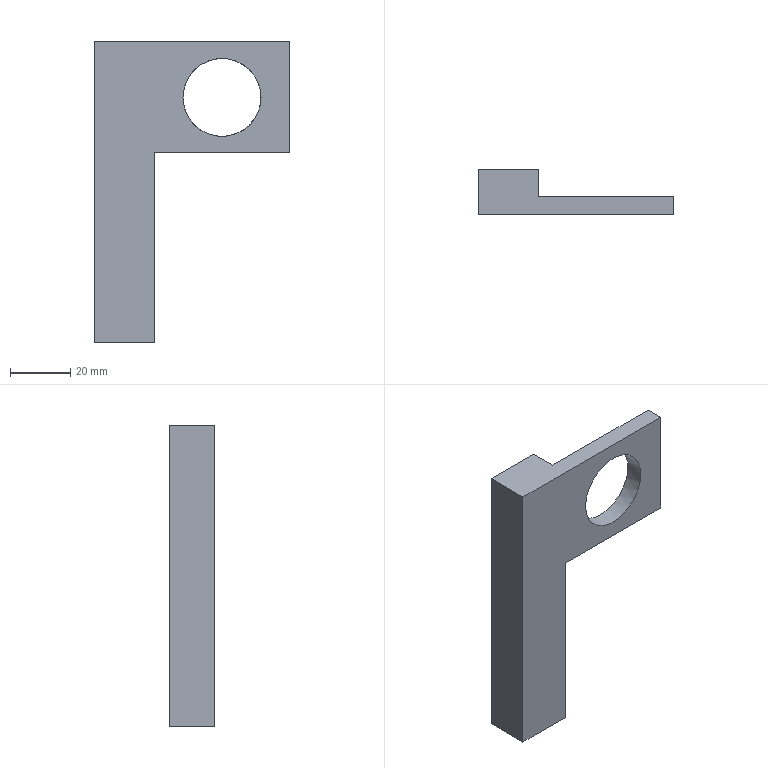Part | STEP file | Tube necking machine_id662_x_t | 1 solid | 10 faces | box 65 x 15 x 100 mm | volume 36804 mm3 | plane 9 | cylinder 1 | commonest cylinder face diameters 26 x1
STEP:
#1=CARTESIAN_POINT('',(0.,0.,0.));
#2=DIRECTION('',(0.,0.,1.));
#3=DIRECTION('',(1.,0.,0.));
#4=AXIS2_PLACEMENT_3D('',#1,#2,#3);
#5=CARTESIAN_POINT('',(240.,-166.,115.5));
#6=VERTEX_POINT('',#5);
#7=CARTESIAN_POINT('',(227.,-166.,128.5));
#8=VERTEX_POINT('',#7);
#9=CARTESIAN_POINT('',(240.,-166.,128.5));
#10=DIRECTION('',(0.,-1.,0.));
#11=DIRECTION('',(0.,0.,-1.));
#12=AXIS2_PLACEMENT_3D('',#9,#10,#11);
#13=CIRCLE('',#12,13.);
#14=CARTESIAN_POINT('',(0.,-166.,0.));
#15=DIRECTION('',(0.,-1.,0.));
#16=DIRECTION('',(0.,0.,-1.));
#17=AXIS2_PLACEMENT_3D('',#14,#15,#16);
#18=PLANE('',#17);
#19=CARTESIAN_POINT('',(-128.5,240.));
#20=DIRECTION('',(1.,0.));
#21=AXIS2_PLACEMENT_2D('',#19,#20);
#22=CIRCLE('',#21,13.);
#23=(GEOMETRIC_REPRESENTATION_CONTEXT(2)PARAMETRIC_REPRESENTATION_CONTEXT()REPRESENTATION_CONTEXT('',''));
#24=DEFINITIONAL_REPRESENTATION('',(#22),#23);
#25=PCURVE('',#18,#24);
#26=CARTESIAN_POINT('',(240.,-172.,128.5));
#27=DIRECTION('',(0.,1.,0.));
#28=DIRECTION('',(0.,0.,1.));
#29=AXIS2_PLACEMENT_3D('',#26,#27,#28);
#30=CYLINDRICAL_SURFACE('',#29,13.);
#31=CARTESIAN_POINT('',(9.425,6.));
#32=DIRECTION('',(-1.,0.));
#33=VECTOR('',#32,1.);
#34=LINE('',#31,#33);
#35=(GEOMETRIC_REPRESENTATION_CONTEXT(2)PARAMETRIC_REPRESENTATION_CONTEXT()REPRESENTATION_CONTEXT('',''));
#36=DEFINITIONAL_REPRESENTATION('',(#34),#35);
#37=PCURVE('',#30,#36);
#38=SURFACE_CURVE('',#13,(#25,#37),.PCURVE_S1.);
#39=EDGE_CURVE('',#6,#8,#38,.T.);
#40=ORIENTED_EDGE('',*,*,#39,.T.);
#41=CARTESIAN_POINT('',(240.,-166.,128.5));
#42=DIRECTION('',(0.,-1.,0.));
#43=DIRECTION('',(0.,0.,-1.));
#44=AXIS2_PLACEMENT_3D('',#41,#42,#43);
#45=CIRCLE('',#44,13.);
#46=CARTESIAN_POINT('',(-128.5,240.));
#47=DIRECTION('',(1.,0.));
#48=AXIS2_PLACEMENT_2D('',#46,#47);
#49=CIRCLE('',#48,13.);
#50=(GEOMETRIC_REPRESENTATION_CONTEXT(2)PARAMETRIC_REPRESENTATION_CONTEXT()REPRESENTATION_CONTEXT('',''));
#51=DEFINITIONAL_REPRESENTATION('',(#49),#50);
#52=PCURVE('',#18,#51);
#53=CARTESIAN_POINT('',(15.708,6.));
#54=DIRECTION('',(-1.,0.));
#55=VECTOR('',#54,1.);
#56=LINE('',#53,#55);
#57=(GEOMETRIC_REPRESENTATION_CONTEXT(2)PARAMETRIC_REPRESENTATION_CONTEXT()REPRESENTATION_CONTEXT('',''));
#58=DEFINITIONAL_REPRESENTATION('',(#56),#57);
#59=PCURVE('',#30,#58);
#60=SURFACE_CURVE('',#45,(#52,#59),.PCURVE_S1.);
#61=EDGE_CURVE('',#8,#6,#60,.T.);
#62=ORIENTED_EDGE('',*,*,#61,.T.);
#63=EDGE_LOOP('',(#40,#62));
#64=FACE_BOUND('',#63,.T.);
#65=CARTESIAN_POINT('',(217.5,-166.,147.));
#66=VERTEX_POINT('',#65);
#67=CARTESIAN_POINT('',(217.5,-166.,110.));
#68=VERTEX_POINT('',#67);
#69=CARTESIAN_POINT('',(217.5,-166.,0.));
#70=DIRECTION('',(0.,0.,-1.));
#71=VECTOR('',#70,1.);
#72=LINE('',#69,#71);
#73=CARTESIAN_POINT('',(0.,217.5));
#74=DIRECTION('',(1.,0.));
#75=VECTOR('',#74,1.);
#76=LINE('',#73,#75);
#77=(GEOMETRIC_REPRESENTATION_CONTEXT(2)PARAMETRIC_REPRESENTATION_CONTEXT()REPRESENTATION_CONTEXT('',''));
#78=DEFINITIONAL_REPRESENTATION('',(#76),#77);
#79=PCURVE('',#18,#78);
#80=CARTESIAN_POINT('',(217.5,-166.,47.));
#81=DIRECTION('',(1.,0.,0.));
#82=DIRECTION('',(0.,0.,-1.));
#83=AXIS2_PLACEMENT_3D('',#80,#81,#82);
#84=PLANE('',#83);
#85=CARTESIAN_POINT('',(47.,0.));
#86=DIRECTION('',(1.,0.));
#87=VECTOR('',#86,1.);
#88=LINE('',#85,#87);
#89=(GEOMETRIC_REPRESENTATION_CONTEXT(2)PARAMETRIC_REPRESENTATION_CONTEXT()REPRESENTATION_CONTEXT('',''));
#90=DEFINITIONAL_REPRESENTATION('',(#88),#89);
#91=PCURVE('',#84,#90);
#92=SURFACE_CURVE('',#72,(#79,#91),.PCURVE_S1.);
#93=EDGE_CURVE('',#66,#68,#92,.T.);
#94=ORIENTED_EDGE('',*,*,#93,.F.);
#95=CARTESIAN_POINT('',(262.5,-166.,147.));
#96=VERTEX_POINT('',#95);
#97=CARTESIAN_POINT('',(262.5,-166.,147.));
#98=DIRECTION('',(-1.,0.,0.));
#99=VECTOR('',#98,1.);
#100=LINE('',#97,#99);
#101=CARTESIAN_POINT('',(-147.,262.5));
#102=DIRECTION('',(0.,-1.));
#103=VECTOR('',#102,1.);
#104=LINE('',#101,#103);
#105=(GEOMETRIC_REPRESENTATION_CONTEXT(2)PARAMETRIC_REPRESENTATION_CONTEXT()REPRESENTATION_CONTEXT('',''));
#106=DEFINITIONAL_REPRESENTATION('',(#104),#105);
#107=PCURVE('',#18,#106);
#108=CARTESIAN_POINT('',(262.5,-166.,147.));
#109=DIRECTION('',(0.,0.,1.));
#110=DIRECTION('',(1.,0.,0.));
#111=AXIS2_PLACEMENT_3D('',#108,#109,#110);
#112=PLANE('',#111);
#113=CARTESIAN_POINT('',(0.,0.));
#114=DIRECTION('',(-1.,0.));
#115=VECTOR('',#114,1.);
#116=LINE('',#113,#115);
#117=(GEOMETRIC_REPRESENTATION_CONTEXT(2)PARAMETRIC_REPRESENTATION_CONTEXT()REPRESENTATION_CONTEXT('',''));
#118=DEFINITIONAL_REPRESENTATION('',(#116),#117);
#119=PCURVE('',#112,#118);
#120=SURFACE_CURVE('',#100,(#107,#119),.PCURVE_S1.);
#121=EDGE_CURVE('',#96,#66,#120,.T.);
#122=ORIENTED_EDGE('',*,*,#121,.F.);
#123=CARTESIAN_POINT('',(262.5,-166.,110.));
#124=VERTEX_POINT('',#123);
#125=CARTESIAN_POINT('',(262.5,-166.,110.));
#126=DIRECTION('',(0.,0.,1.));
#127=VECTOR('',#126,1.);
#128=LINE('',#125,#127);
#129=CARTESIAN_POINT('',(-110.,262.5));
#130=DIRECTION('',(-1.,0.));
#131=VECTOR('',#130,1.);
#132=LINE('',#129,#131);
#133=(GEOMETRIC_REPRESENTATION_CONTEXT(2)PARAMETRIC_REPRESENTATION_CONTEXT()REPRESENTATION_CONTEXT('',''));
#134=DEFINITIONAL_REPRESENTATION('',(#132),#133);
#135=PCURVE('',#18,#134);
#136=CARTESIAN_POINT('',(262.5,-166.,110.));
#137=DIRECTION('',(1.,0.,0.));
#138=DIRECTION('',(0.,0.,-1.));
#139=AXIS2_PLACEMENT_3D('',#136,#137,#138);
#140=PLANE('',#139);
#141=CARTESIAN_POINT('',(0.,0.));
#142=DIRECTION('',(-1.,0.));
#143=VECTOR('',#142,1.);
#144=LINE('',#141,#143);
#145=(GEOMETRIC_REPRESENTATION_CONTEXT(2)PARAMETRIC_REPRESENTATION_CONTEXT()REPRESENTATION_CONTEXT('',''));
#146=DEFINITIONAL_REPRESENTATION('',(#144),#145);
#147=PCURVE('',#140,#146);
#148=SURFACE_CURVE('',#128,(#135,#147),.PCURVE_S1.);
#149=EDGE_CURVE('',#124,#96,#148,.T.);
#150=ORIENTED_EDGE('',*,*,#149,.F.);
#151=CARTESIAN_POINT('',(217.5,-166.,110.));
#152=DIRECTION('',(1.,0.,0.));
#153=VECTOR('',#152,1.);
#154=LINE('',#151,#153);
#155=CARTESIAN_POINT('',(-110.,217.5));
#156=DIRECTION('',(0.,1.));
#157=VECTOR('',#156,1.);
#158=LINE('',#155,#157);
#159=(GEOMETRIC_REPRESENTATION_CONTEXT(2)PARAMETRIC_REPRESENTATION_CONTEXT()REPRESENTATION_CONTEXT('',''));
#160=DEFINITIONAL_REPRESENTATION('',(#158),#159);
#161=PCURVE('',#18,#160);
#162=CARTESIAN_POINT('',(217.5,-166.,110.));
#163=DIRECTION('',(0.,0.,-1.));
#164=DIRECTION('',(-1.,0.,0.));
#165=AXIS2_PLACEMENT_3D('',#162,#163,#164);
#166=PLANE('',#165);
#167=CARTESIAN_POINT('',(0.,0.));
#168=DIRECTION('',(-1.,0.));
#169=VECTOR('',#168,1.);
#170=LINE('',#167,#169);
#171=(GEOMETRIC_REPRESENTATION_CONTEXT(2)PARAMETRIC_REPRESENTATION_CONTEXT()REPRESENTATION_CONTEXT('',''));
#172=DEFINITIONAL_REPRESENTATION('',(#170),#171);
#173=PCURVE('',#166,#172);
#174=SURFACE_CURVE('',#154,(#161,#173),.PCURVE_S1.);
#175=EDGE_CURVE('',#68,#124,#174,.T.);
#176=ORIENTED_EDGE('',*,*,#175,.F.);
#177=EDGE_LOOP('',(#94,#122,#150,#176));
#178=FACE_BOUND('',#177,.T.);
#179=ADVANCED_FACE('',(#64,#178),#18,.F.);
#180=CARTESIAN_POINT('',(197.5,-172.,147.));
#181=VERTEX_POINT('',#180);
#182=CARTESIAN_POINT('',(197.5,-172.,47.));
#183=VERTEX_POINT('',#182);
#184=CARTESIAN_POINT('',(197.5,-172.,147.));
#185=DIRECTION('',(0.,0.,-1.));
#186=VECTOR('',#185,1.);
#187=LINE('',#184,#186);
#188=CARTESIAN_POINT('',(197.5,-166.,147.));
#189=DIRECTION('',(-1.,0.,0.));
#190=DIRECTION('',(0.,0.,1.));
#191=AXIS2_PLACEMENT_3D('',#188,#189,#190);
#192=PLANE('',#191);
#193=CARTESIAN_POINT('',(0.,-6.));
#194=DIRECTION('',(-1.,0.));
#195=VECTOR('',#194,1.);
#196=LINE('',#193,#195);
#197=(GEOMETRIC_REPRESENTATION_CONTEXT(2)PARAMETRIC_REPRESENTATION_CONTEXT()REPRESENTATION_CONTEXT('',''));
#198=DEFINITIONAL_REPRESENTATION('',(#196),#197);
#199=PCURVE('',#192,#198);
#200=CARTESIAN_POINT('',(0.,-172.,0.));
#201=DIRECTION('',(0.,-1.,0.));
#202=DIRECTION('',(0.,0.,-1.));
#203=AXIS2_PLACEMENT_3D('',#200,#201,#202);
#204=PLANE('',#203);
#205=CARTESIAN_POINT('',(-147.,197.5));
#206=DIRECTION('',(1.,0.));
#207=VECTOR('',#206,1.);
#208=LINE('',#205,#207);
#209=(GEOMETRIC_REPRESENTATION_CONTEXT(2)PARAMETRIC_REPRESENTATION_CONTEXT()REPRESENTATION_CONTEXT('',''));
#210=DEFINITIONAL_REPRESENTATION('',(#208),#209);
#211=PCURVE('',#204,#210);
#212=SURFACE_CURVE('',#187,(#199,#211),.PCURVE_S1.);
#213=EDGE_CURVE('',#181,#183,#212,.T.);
#214=ORIENTED_EDGE('',*,*,#213,.F.);
#215=CARTESIAN_POINT('',(197.5,-157.,147.));
#216=VERTEX_POINT('',#215);
#217=CARTESIAN_POINT('',(197.5,-166.,147.));
#218=DIRECTION('',(0.,-1.,0.));
#219=VECTOR('',#218,1.);
#220=LINE('',#217,#219);
#221=CARTESIAN_POINT('',(0.,0.));
#222=DIRECTION('',(0.,-1.));
#223=VECTOR('',#222,1.);
#224=LINE('',#221,#223);
#225=(GEOMETRIC_REPRESENTATION_CONTEXT(2)PARAMETRIC_REPRESENTATION_CONTEXT()REPRESENTATION_CONTEXT('',''));
#226=DEFINITIONAL_REPRESENTATION('',(#224),#225);
#227=PCURVE('',#192,#226);
#228=CARTESIAN_POINT('',(-65.,0.));
#229=DIRECTION('',(0.,-1.));
#230=VECTOR('',#229,1.);
#231=LINE('',#228,#230);
#232=(GEOMETRIC_REPRESENTATION_CONTEXT(2)PARAMETRIC_REPRESENTATION_CONTEXT()REPRESENTATION_CONTEXT('',''));
#233=DEFINITIONAL_REPRESENTATION('',(#231),#232);
#234=PCURVE('',#112,#233);
#235=SURFACE_CURVE('',#220,(#227,#234),.PCURVE_S1.);
#236=EDGE_CURVE('',#216,#181,#235,.T.);
#237=ORIENTED_EDGE('',*,*,#236,.F.);
#238=CARTESIAN_POINT('',(197.5,-157.,47.));
#239=VERTEX_POINT('',#238);
#240=CARTESIAN_POINT('',(197.5,-157.,147.));
#241=DIRECTION('',(0.,0.,-1.));
#242=VECTOR('',#241,1.);
#243=LINE('',#240,#242);
#244=CARTESIAN_POINT('',(0.,9.));
#245=DIRECTION('',(-1.,0.));
#246=VECTOR('',#245,1.);
#247=LINE('',#244,#246);
#248=(GEOMETRIC_REPRESENTATION_CONTEXT(2)PARAMETRIC_REPRESENTATION_CONTEXT()REPRESENTATION_CONTEXT('',''));
#249=DEFINITIONAL_REPRESENTATION('',(#247),#248);
#250=PCURVE('',#192,#249);
#251=CARTESIAN_POINT('',(197.5,-157.,147.));
#252=DIRECTION('',(0.,1.,0.));
#253=DIRECTION('',(0.,0.,-1.));
#254=AXIS2_PLACEMENT_3D('',#251,#252,#253);
#255=PLANE('',#254);
#256=CARTESIAN_POINT('',(0.,0.));
#257=DIRECTION('',(1.,0.));
#258=VECTOR('',#257,1.);
#259=LINE('',#256,#258);
#260=(GEOMETRIC_REPRESENTATION_CONTEXT(2)PARAMETRIC_REPRESENTATION_CONTEXT()REPRESENTATION_CONTEXT('',''));
#261=DEFINITIONAL_REPRESENTATION('',(#259),#260);
#262=PCURVE('',#255,#261);
#263=SURFACE_CURVE('',#243,(#250,#262),.PCURVE_S1.);
#264=EDGE_CURVE('',#216,#239,#263,.T.);
#265=ORIENTED_EDGE('',*,*,#264,.T.);
#266=CARTESIAN_POINT('',(197.5,-166.,47.));
#267=DIRECTION('',(0.,-1.,0.));
#268=VECTOR('',#267,1.);
#269=LINE('',#266,#268);
#270=CARTESIAN_POINT('',(-100.,0.));
#271=DIRECTION('',(0.,-1.));
#272=VECTOR('',#271,1.);
#273=LINE('',#270,#272);
#274=(GEOMETRIC_REPRESENTATION_CONTEXT(2)PARAMETRIC_REPRESENTATION_CONTEXT()REPRESENTATION_CONTEXT('',''));
#275=DEFINITIONAL_REPRESENTATION('',(#273),#274);
#276=PCURVE('',#192,#275);
#277=CARTESIAN_POINT('',(197.5,-166.,47.));
#278=DIRECTION('',(0.,0.,-1.));
#279=DIRECTION('',(-1.,0.,0.));
#280=AXIS2_PLACEMENT_3D('',#277,#278,#279);
#281=PLANE('',#280);
#282=CARTESIAN_POINT('',(0.,0.));
#283=DIRECTION('',(0.,-1.));
#284=VECTOR('',#283,1.);
#285=LINE('',#282,#284);
#286=(GEOMETRIC_REPRESENTATION_CONTEXT(2)PARAMETRIC_REPRESENTATION_CONTEXT()REPRESENTATION_CONTEXT('',''));
#287=DEFINITIONAL_REPRESENTATION('',(#285),#286);
#288=PCURVE('',#281,#287);
#289=SURFACE_CURVE('',#269,(#276,#288),.PCURVE_S1.);
#290=EDGE_CURVE('',#239,#183,#289,.T.);
#291=ORIENTED_EDGE('',*,*,#290,.T.);
#292=EDGE_LOOP('',(#214,#237,#265,#291));
#293=FACE_BOUND('',#292,.T.);
#294=ADVANCED_FACE('',(#293),#192,.T.);
#295=CARTESIAN_POINT('',(217.5,-172.,47.));
#296=VERTEX_POINT('',#295);
#297=CARTESIAN_POINT('',(197.5,-172.,47.));
#298=DIRECTION('',(1.,0.,0.));
#299=VECTOR('',#298,1.);
#300=LINE('',#297,#299);
#301=CARTESIAN_POINT('',(0.,-6.));
#302=DIRECTION('',(-1.,0.));
#303=VECTOR('',#302,1.);
#304=LINE('',#301,#303);
#305=(GEOMETRIC_REPRESENTATION_CONTEXT(2)PARAMETRIC_REPRESENTATION_CONTEXT()REPRESENTATION_CONTEXT('',''));
#306=DEFINITIONAL_REPRESENTATION('',(#304),#305);
#307=PCURVE('',#281,#306);
#308=CARTESIAN_POINT('',(-47.,197.5));
#309=DIRECTION('',(0.,1.));
#310=VECTOR('',#309,1.);
#311=LINE('',#308,#310);
#312=(GEOMETRIC_REPRESENTATION_CONTEXT(2)PARAMETRIC_REPRESENTATION_CONTEXT()REPRESENTATION_CONTEXT('',''));
#313=DEFINITIONAL_REPRESENTATION('',(#311),#312);
#314=PCURVE('',#204,#313);
#315=SURFACE_CURVE('',#300,(#307,#314),.PCURVE_S1.);
#316=EDGE_CURVE('',#183,#296,#315,.T.);
#317=ORIENTED_EDGE('',*,*,#316,.F.);
#318=ORIENTED_EDGE('',*,*,#290,.F.);
#319=CARTESIAN_POINT('',(217.5,-157.,47.));
#320=VERTEX_POINT('',#319);
#321=CARTESIAN_POINT('',(197.5,-157.,47.));
#322=DIRECTION('',(1.,0.,0.));
#323=VECTOR('',#322,1.);
#324=LINE('',#321,#323);
#325=CARTESIAN_POINT('',(0.,9.));
#326=DIRECTION('',(-1.,0.));
#327=VECTOR('',#326,1.);
#328=LINE('',#325,#327);
#329=(GEOMETRIC_REPRESENTATION_CONTEXT(2)PARAMETRIC_REPRESENTATION_CONTEXT()REPRESENTATION_CONTEXT('',''));
#330=DEFINITIONAL_REPRESENTATION('',(#328),#329);
#331=PCURVE('',#281,#330);
#332=CARTESIAN_POINT('',(100.,0.));
#333=DIRECTION('',(0.,-1.));
#334=VECTOR('',#333,1.);
#335=LINE('',#332,#334);
#336=(GEOMETRIC_REPRESENTATION_CONTEXT(2)PARAMETRIC_REPRESENTATION_CONTEXT()REPRESENTATION_CONTEXT('',''));
#337=DEFINITIONAL_REPRESENTATION('',(#335),#336);
#338=PCURVE('',#255,#337);
#339=SURFACE_CURVE('',#324,(#331,#338),.PCURVE_S1.);
#340=EDGE_CURVE('',#239,#320,#339,.T.);
#341=ORIENTED_EDGE('',*,*,#340,.T.);
#342=CARTESIAN_POINT('',(217.5,-166.,47.));
#343=DIRECTION('',(0.,-1.,0.));
#344=VECTOR('',#343,1.);
#345=LINE('',#342,#344);
#346=CARTESIAN_POINT('',(-20.,0.));
#347=DIRECTION('',(0.,-1.));
#348=VECTOR('',#347,1.);
#349=LINE('',#346,#348);
#350=(GEOMETRIC_REPRESENTATION_CONTEXT(2)PARAMETRIC_REPRESENTATION_CONTEXT()REPRESENTATION_CONTEXT('',''));
#351=DEFINITIONAL_REPRESENTATION('',(#349),#350);
#352=PCURVE('',#281,#351);
#353=CARTESIAN_POINT('',(0.,0.));
#354=DIRECTION('',(0.,-1.));
#355=VECTOR('',#354,1.);
#356=LINE('',#353,#355);
#357=(GEOMETRIC_REPRESENTATION_CONTEXT(2)PARAMETRIC_REPRESENTATION_CONTEXT()REPRESENTATION_CONTEXT('',''));
#358=DEFINITIONAL_REPRESENTATION('',(#356),#357);
#359=PCURVE('',#84,#358);
#360=SURFACE_CURVE('',#345,(#352,#359),.PCURVE_S1.);
#361=EDGE_CURVE('',#320,#296,#360,.T.);
#362=ORIENTED_EDGE('',*,*,#361,.T.);
#363=EDGE_LOOP('',(#317,#318,#341,#362));
#364=FACE_BOUND('',#363,.T.);
#365=ADVANCED_FACE('',(#364),#281,.T.);
#366=CARTESIAN_POINT('',(217.5,-172.,110.));
#367=VERTEX_POINT('',#366);
#368=CARTESIAN_POINT('',(217.5,-172.,47.));
#369=DIRECTION('',(0.,0.,1.));
#370=VECTOR('',#369,1.);
#371=LINE('',#368,#370);
#372=CARTESIAN_POINT('',(0.,-6.));
#373=DIRECTION('',(-1.,0.));
#374=VECTOR('',#373,1.);
#375=LINE('',#372,#374);
#376=(GEOMETRIC_REPRESENTATION_CONTEXT(2)PARAMETRIC_REPRESENTATION_CONTEXT()REPRESENTATION_CONTEXT('',''));
#377=DEFINITIONAL_REPRESENTATION('',(#375),#376);
#378=PCURVE('',#84,#377);
#379=CARTESIAN_POINT('',(-47.,217.5));
#380=DIRECTION('',(-1.,0.));
#381=VECTOR('',#380,1.);
#382=LINE('',#379,#381);
#383=(GEOMETRIC_REPRESENTATION_CONTEXT(2)PARAMETRIC_REPRESENTATION_CONTEXT()REPRESENTATION_CONTEXT('',''));
#384=DEFINITIONAL_REPRESENTATION('',(#382),#383);
#385=PCURVE('',#204,#384);
#386=SURFACE_CURVE('',#371,(#378,#385),.PCURVE_S1.);
#387=EDGE_CURVE('',#296,#367,#386,.T.);
#388=ORIENTED_EDGE('',*,*,#387,.F.);
#389=ORIENTED_EDGE('',*,*,#361,.F.);
#390=CARTESIAN_POINT('',(217.5,-157.,147.));
#391=VERTEX_POINT('',#390);
#392=CARTESIAN_POINT('',(217.5,-157.,147.));
#393=DIRECTION('',(0.,0.,-1.));
#394=VECTOR('',#393,1.);
#395=LINE('',#392,#394);
#396=CARTESIAN_POINT('',(-100.,9.));
#397=DIRECTION('',(1.,0.));
#398=VECTOR('',#397,1.);
#399=LINE('',#396,#398);
#400=(GEOMETRIC_REPRESENTATION_CONTEXT(2)PARAMETRIC_REPRESENTATION_CONTEXT()REPRESENTATION_CONTEXT('',''));
#401=DEFINITIONAL_REPRESENTATION('',(#399),#400);
#402=PCURVE('',#84,#401);
#403=CARTESIAN_POINT('',(0.,-20.));
#404=DIRECTION('',(1.,0.));
#405=VECTOR('',#404,1.);
#406=LINE('',#403,#405);
#407=(GEOMETRIC_REPRESENTATION_CONTEXT(2)PARAMETRIC_REPRESENTATION_CONTEXT()REPRESENTATION_CONTEXT('',''));
#408=DEFINITIONAL_REPRESENTATION('',(#406),#407);
#409=PCURVE('',#255,#408);
#410=SURFACE_CURVE('',#395,(#402,#409),.PCURVE_S1.);
#411=EDGE_CURVE('',#391,#320,#410,.T.);
#412=ORIENTED_EDGE('',*,*,#411,.F.);
#413=CARTESIAN_POINT('',(217.5,-157.,147.));
#414=DIRECTION('',(0.,-1.,0.));
#415=VECTOR('',#414,1.);
#416=LINE('',#413,#415);
#417=CARTESIAN_POINT('',(-100.,9.));
#418=DIRECTION('',(0.,-1.));
#419=VECTOR('',#418,1.);
#420=LINE('',#417,#419);
#421=(GEOMETRIC_REPRESENTATION_CONTEXT(2)PARAMETRIC_REPRESENTATION_CONTEXT()REPRESENTATION_CONTEXT('',''));
#422=DEFINITIONAL_REPRESENTATION('',(#420),#421);
#423=PCURVE('',#84,#422);
#424=CARTESIAN_POINT('',(-45.,9.));
#425=DIRECTION('',(0.,-1.));
#426=VECTOR('',#425,1.);
#427=LINE('',#424,#426);
#428=(GEOMETRIC_REPRESENTATION_CONTEXT(2)PARAMETRIC_REPRESENTATION_CONTEXT()REPRESENTATION_CONTEXT('',''));
#429=DEFINITIONAL_REPRESENTATION('',(#427),#428);
#430=PCURVE('',#112,#429);
#431=SURFACE_CURVE('',#416,(#423,#430),.PCURVE_S1.);
#432=EDGE_CURVE('',#391,#66,#431,.T.);
#433=ORIENTED_EDGE('',*,*,#432,.T.);
#434=ORIENTED_EDGE('',*,*,#93,.T.);
#435=CARTESIAN_POINT('',(217.5,-166.,110.));
#436=DIRECTION('',(0.,-1.,0.));
#437=VECTOR('',#436,1.);
#438=LINE('',#435,#437);
#439=CARTESIAN_POINT('',(-63.,0.));
#440=DIRECTION('',(0.,-1.));
#441=VECTOR('',#440,1.);
#442=LINE('',#439,#441);
#443=(GEOMETRIC_REPRESENTATION_CONTEXT(2)PARAMETRIC_REPRESENTATION_CONTEXT()REPRESENTATION_CONTEXT('',''));
#444=DEFINITIONAL_REPRESENTATION('',(#442),#443);
#445=PCURVE('',#84,#444);
#446=CARTESIAN_POINT('',(0.,0.));
#447=DIRECTION('',(0.,-1.));
#448=VECTOR('',#447,1.);
#449=LINE('',#446,#448);
#450=(GEOMETRIC_REPRESENTATION_CONTEXT(2)PARAMETRIC_REPRESENTATION_CONTEXT()REPRESENTATION_CONTEXT('',''));
#451=DEFINITIONAL_REPRESENTATION('',(#449),#450);
#452=PCURVE('',#166,#451);
#453=SURFACE_CURVE('',#438,(#445,#452),.PCURVE_S1.);
#454=EDGE_CURVE('',#68,#367,#453,.T.);
#455=ORIENTED_EDGE('',*,*,#454,.T.);
#456=EDGE_LOOP('',(#388,#389,#412,#433,#434,#455));
#457=FACE_BOUND('',#456,.T.);
#458=ADVANCED_FACE('',(#457),#84,.T.);
#459=CARTESIAN_POINT('',(262.5,-172.,110.));
#460=VERTEX_POINT('',#459);
#461=CARTESIAN_POINT('',(217.5,-172.,110.));
#462=DIRECTION('',(1.,0.,0.));
#463=VECTOR('',#462,1.);
#464=LINE('',#461,#463);
#465=CARTESIAN_POINT('',(0.,-6.));
#466=DIRECTION('',(-1.,0.));
#467=VECTOR('',#466,1.);
#468=LINE('',#465,#467);
#469=(GEOMETRIC_REPRESENTATION_CONTEXT(2)PARAMETRIC_REPRESENTATION_CONTEXT()REPRESENTATION_CONTEXT('',''));
#470=DEFINITIONAL_REPRESENTATION('',(#468),#469);
#471=PCURVE('',#166,#470);
#472=CARTESIAN_POINT('',(-110.,217.5));
#473=DIRECTION('',(0.,1.));
#474=VECTOR('',#473,1.);
#475=LINE('',#472,#474);
#476=(GEOMETRIC_REPRESENTATION_CONTEXT(2)PARAMETRIC_REPRESENTATION_CONTEXT()REPRESENTATION_CONTEXT('',''));
#477=DEFINITIONAL_REPRESENTATION('',(#475),#476);
#478=PCURVE('',#204,#477);
#479=SURFACE_CURVE('',#464,(#471,#478),.PCURVE_S1.);
#480=EDGE_CURVE('',#367,#460,#479,.T.);
#481=ORIENTED_EDGE('',*,*,#480,.F.);
#482=ORIENTED_EDGE('',*,*,#454,.F.);
#483=ORIENTED_EDGE('',*,*,#175,.T.);
#484=CARTESIAN_POINT('',(262.5,-166.,110.));
#485=DIRECTION('',(0.,-1.,0.));
#486=VECTOR('',#485,1.);
#487=LINE('',#484,#486);
#488=CARTESIAN_POINT('',(-45.,0.));
#489=DIRECTION('',(0.,-1.));
#490=VECTOR('',#489,1.);
#491=LINE('',#488,#490);
#492=(GEOMETRIC_REPRESENTATION_CONTEXT(2)PARAMETRIC_REPRESENTATION_CONTEXT()REPRESENTATION_CONTEXT('',''));
#493=DEFINITIONAL_REPRESENTATION('',(#491),#492);
#494=PCURVE('',#166,#493);
#495=CARTESIAN_POINT('',(0.,0.));
#496=DIRECTION('',(0.,-1.));
#497=VECTOR('',#496,1.);
#498=LINE('',#495,#497);
#499=(GEOMETRIC_REPRESENTATION_CONTEXT(2)PARAMETRIC_REPRESENTATION_CONTEXT()REPRESENTATION_CONTEXT('',''));
#500=DEFINITIONAL_REPRESENTATION('',(#498),#499);
#501=PCURVE('',#140,#500);
#502=SURFACE_CURVE('',#487,(#494,#501),.PCURVE_S1.);
#503=EDGE_CURVE('',#124,#460,#502,.T.);
#504=ORIENTED_EDGE('',*,*,#503,.T.);
#505=EDGE_LOOP('',(#481,#482,#483,#504));
#506=FACE_BOUND('',#505,.T.);
#507=ADVANCED_FACE('',(#506),#166,.T.);
#508=CARTESIAN_POINT('',(262.5,-172.,147.));
#509=VERTEX_POINT('',#508);
#510=CARTESIAN_POINT('',(262.5,-172.,110.));
#511=DIRECTION('',(0.,0.,1.));
#512=VECTOR('',#511,1.);
#513=LINE('',#510,#512);
#514=CARTESIAN_POINT('',(0.,-6.));
#515=DIRECTION('',(-1.,0.));
#516=VECTOR('',#515,1.);
#517=LINE('',#514,#516);
#518=(GEOMETRIC_REPRESENTATION_CONTEXT(2)PARAMETRIC_REPRESENTATION_CONTEXT()REPRESENTATION_CONTEXT('',''));
#519=DEFINITIONAL_REPRESENTATION('',(#517),#518);
#520=PCURVE('',#140,#519);
#521=CARTESIAN_POINT('',(-110.,262.5));
#522=DIRECTION('',(-1.,0.));
#523=VECTOR('',#522,1.);
#524=LINE('',#521,#523);
#525=(GEOMETRIC_REPRESENTATION_CONTEXT(2)PARAMETRIC_REPRESENTATION_CONTEXT()REPRESENTATION_CONTEXT('',''));
#526=DEFINITIONAL_REPRESENTATION('',(#524),#525);
#527=PCURVE('',#204,#526);
#528=SURFACE_CURVE('',#513,(#520,#527),.PCURVE_S1.);
#529=EDGE_CURVE('',#460,#509,#528,.T.);
#530=ORIENTED_EDGE('',*,*,#529,.F.);
#531=ORIENTED_EDGE('',*,*,#503,.F.);
#532=ORIENTED_EDGE('',*,*,#149,.T.);
#533=CARTESIAN_POINT('',(262.5,-166.,147.));
#534=DIRECTION('',(0.,-1.,0.));
#535=VECTOR('',#534,1.);
#536=LINE('',#533,#535);
#537=CARTESIAN_POINT('',(-37.,0.));
#538=DIRECTION('',(0.,-1.));
#539=VECTOR('',#538,1.);
#540=LINE('',#537,#539);
#541=(GEOMETRIC_REPRESENTATION_CONTEXT(2)PARAMETRIC_REPRESENTATION_CONTEXT()REPRESENTATION_CONTEXT('',''));
#542=DEFINITIONAL_REPRESENTATION('',(#540),#541);
#543=PCURVE('',#140,#542);
#544=CARTESIAN_POINT('',(0.,0.));
#545=DIRECTION('',(0.,-1.));
#546=VECTOR('',#545,1.);
#547=LINE('',#544,#546);
#548=(GEOMETRIC_REPRESENTATION_CONTEXT(2)PARAMETRIC_REPRESENTATION_CONTEXT()REPRESENTATION_CONTEXT('',''));
#549=DEFINITIONAL_REPRESENTATION('',(#547),#548);
#550=PCURVE('',#112,#549);
#551=SURFACE_CURVE('',#536,(#543,#550),.PCURVE_S1.);
#552=EDGE_CURVE('',#96,#509,#551,.T.);
#553=ORIENTED_EDGE('',*,*,#552,.T.);
#554=EDGE_LOOP('',(#530,#531,#532,#553));
#555=FACE_BOUND('',#554,.T.);
#556=ADVANCED_FACE('',(#555),#140,.T.);
#557=ORIENTED_EDGE('',*,*,#236,.T.);
#558=CARTESIAN_POINT('',(262.5,-172.,147.));
#559=DIRECTION('',(-1.,0.,0.));
#560=VECTOR('',#559,1.);
#561=LINE('',#558,#560);
#562=CARTESIAN_POINT('',(0.,-6.));
#563=DIRECTION('',(-1.,0.));
#564=VECTOR('',#563,1.);
#565=LINE('',#562,#564);
#566=(GEOMETRIC_REPRESENTATION_CONTEXT(2)PARAMETRIC_REPRESENTATION_CONTEXT()REPRESENTATION_CONTEXT('',''));
#567=DEFINITIONAL_REPRESENTATION('',(#565),#566);
#568=PCURVE('',#112,#567);
#569=CARTESIAN_POINT('',(-147.,262.5));
#570=DIRECTION('',(0.,-1.));
#571=VECTOR('',#570,1.);
#572=LINE('',#569,#571);
#573=(GEOMETRIC_REPRESENTATION_CONTEXT(2)PARAMETRIC_REPRESENTATION_CONTEXT()REPRESENTATION_CONTEXT('',''));
#574=DEFINITIONAL_REPRESENTATION('',(#572),#573);
#575=PCURVE('',#204,#574);
#576=SURFACE_CURVE('',#561,(#568,#575),.PCURVE_S1.);
#577=EDGE_CURVE('',#509,#181,#576,.T.);
#578=ORIENTED_EDGE('',*,*,#577,.F.);
#579=ORIENTED_EDGE('',*,*,#552,.F.);
#580=ORIENTED_EDGE('',*,*,#121,.T.);
#581=ORIENTED_EDGE('',*,*,#432,.F.);
#582=CARTESIAN_POINT('',(197.5,-157.,147.));
#583=DIRECTION('',(1.,0.,0.));
#584=VECTOR('',#583,1.);
#585=LINE('',#582,#584);
#586=CARTESIAN_POINT('',(-65.,9.));
#587=DIRECTION('',(1.,0.));
#588=VECTOR('',#587,1.);
#589=LINE('',#586,#588);
#590=(GEOMETRIC_REPRESENTATION_CONTEXT(2)PARAMETRIC_REPRESENTATION_CONTEXT()REPRESENTATION_CONTEXT('',''));
#591=DEFINITIONAL_REPRESENTATION('',(#589),#590);
#592=PCURVE('',#112,#591);
#593=CARTESIAN_POINT('',(0.,0.));
#594=DIRECTION('',(0.,-1.));
#595=VECTOR('',#594,1.);
#596=LINE('',#593,#595);
#597=(GEOMETRIC_REPRESENTATION_CONTEXT(2)PARAMETRIC_REPRESENTATION_CONTEXT()REPRESENTATION_CONTEXT('',''));
#598=DEFINITIONAL_REPRESENTATION('',(#596),#597);
#599=PCURVE('',#255,#598);
#600=SURFACE_CURVE('',#585,(#592,#599),.PCURVE_S1.);
#601=EDGE_CURVE('',#216,#391,#600,.T.);
#602=ORIENTED_EDGE('',*,*,#601,.F.);
#603=EDGE_LOOP('',(#557,#578,#579,#580,#581,#602));
#604=FACE_BOUND('',#603,.T.);
#605=ADVANCED_FACE('',(#604),#112,.T.);
#606=CARTESIAN_POINT('',(227.,-172.,128.5));
#607=VERTEX_POINT('',#606);
#608=CARTESIAN_POINT('',(240.,-172.,128.5));
#609=DIRECTION('',(0.,1.,0.));
#610=DIRECTION('',(-1.,0.,0.));
#611=AXIS2_PLACEMENT_3D('',#608,#609,#610);
#612=CIRCLE('',#611,13.);
#613=CARTESIAN_POINT('',(-128.5,227.));
#614=CARTESIAN_POINT('',(-151.017,227.));
#615=CARTESIAN_POINT('',(-139.758,246.5));
#616=CARTESIAN_POINT('',(-128.5,266.));
#617=CARTESIAN_POINT('',(-117.242,246.5));
#618=CARTESIAN_POINT('',(-105.983,227.));
#619=CARTESIAN_POINT('',(-128.5,227.));
#620=(BOUNDED_CURVE()B_SPLINE_CURVE(2,(#613,#614,#615,#616,#617,#618,#619),.UNSPECIFIED.,.T.,.F.)B_SPLINE_CURVE_WITH_KNOTS((1,2,2,2,2,1),(-2.094,0.,2.094,4.189,6.283,8.378),.UNSPECIFIED.)CURVE()GEOMETRIC_REPRESENTATION_ITEM()RATIONAL_B_SPLINE_CURVE((1.,0.5,1.,0.5,1.,0.5,1.))REPRESENTATION_ITEM(''));
#621=(GEOMETRIC_REPRESENTATION_CONTEXT(2)PARAMETRIC_REPRESENTATION_CONTEXT()REPRESENTATION_CONTEXT('',''));
#622=DEFINITIONAL_REPRESENTATION('',(#620),#621);
#623=PCURVE('',#204,#622);
#624=CARTESIAN_POINT('',(4.712,0.));
#625=DIRECTION('',(1.,0.));
#626=VECTOR('',#625,1.);
#627=LINE('',#624,#626);
#628=(GEOMETRIC_REPRESENTATION_CONTEXT(2)PARAMETRIC_REPRESENTATION_CONTEXT()REPRESENTATION_CONTEXT('',''));
#629=DEFINITIONAL_REPRESENTATION('',(#627),#628);
#630=PCURVE('',#30,#629);
#631=SURFACE_CURVE('',#612,(#623,#630),.PCURVE_S1.);
#632=EDGE_CURVE('',#607,#607,#631,.T.);
#633=ORIENTED_EDGE('',*,*,#632,.T.);
#634=EDGE_LOOP('',(#633));
#635=FACE_BOUND('',#634,.T.);
#636=ORIENTED_EDGE('',*,*,#387,.T.);
#637=ORIENTED_EDGE('',*,*,#480,.T.);
#638=ORIENTED_EDGE('',*,*,#529,.T.);
#639=ORIENTED_EDGE('',*,*,#577,.T.);
#640=ORIENTED_EDGE('',*,*,#213,.T.);
#641=ORIENTED_EDGE('',*,*,#316,.T.);
#642=EDGE_LOOP('',(#636,#637,#638,#639,#640,#641));
#643=FACE_BOUND('',#642,.T.);
#644=ADVANCED_FACE('',(#635,#643),#204,.T.);
#645=ORIENTED_EDGE('',*,*,#340,.F.);
#646=ORIENTED_EDGE('',*,*,#264,.F.);
#647=ORIENTED_EDGE('',*,*,#601,.T.);
#648=ORIENTED_EDGE('',*,*,#411,.T.);
#649=EDGE_LOOP('',(#645,#646,#647,#648));
#650=FACE_BOUND('',#649,.T.);
#651=ADVANCED_FACE('',(#650),#255,.T.);
#652=ORIENTED_EDGE('',*,*,#632,.T.);
#653=CARTESIAN_POINT('',(227.,-172.,128.5));
#654=CARTESIAN_POINT('',(227.,-166.,128.5));
#655=B_SPLINE_CURVE_WITH_KNOTS('',1,(#653,#654),.UNSPECIFIED.,.F.,.F.,(2,2),(0.,6.),.PIECEWISE_BEZIER_KNOTS.);
#656=CARTESIAN_POINT('',(10.996,0.));
#657=DIRECTION('',(0.,1.));
#658=VECTOR('',#657,1.);
#659=LINE('',#656,#658);
#660=(GEOMETRIC_REPRESENTATION_CONTEXT(2)PARAMETRIC_REPRESENTATION_CONTEXT()REPRESENTATION_CONTEXT('',''));
#661=DEFINITIONAL_REPRESENTATION('',(#659),#660);
#662=PCURVE('',#30,#661);
#663=CARTESIAN_POINT('',(4.712,0.));
#664=DIRECTION('',(0.,1.));
#665=VECTOR('',#664,1.);
#666=LINE('',#663,#665);
#667=(GEOMETRIC_REPRESENTATION_CONTEXT(2)PARAMETRIC_REPRESENTATION_CONTEXT()REPRESENTATION_CONTEXT('',''));
#668=DEFINITIONAL_REPRESENTATION('',(#666),#667);
#669=PCURVE('',#30,#668);
#670=SEAM_CURVE('',#655,(#662,#669),.PCURVE_S1.);
#671=EDGE_CURVE('',#607,#8,#670,.T.);
#672=ORIENTED_EDGE('',*,*,#671,.T.);
#673=ORIENTED_EDGE('',*,*,#61,.T.);
#674=ORIENTED_EDGE('',*,*,#39,.T.);
#675=ORIENTED_EDGE('',*,*,#671,.F.);
#676=EDGE_LOOP('',(#652,#672,#673,#674,#675));
#677=FACE_BOUND('',#676,.F.);
#678=ADVANCED_FACE('',(#677),#30,.F.);
#679=CLOSED_SHELL('',(#179,#294,#365,#458,#507,#556,#605,#644,#651,#678));
#680=MANIFOLD_SOLID_BREP('',#679);
#681=(LENGTH_UNIT()NAMED_UNIT(*)SI_UNIT(.MILLI.,.METRE.));
#682=UNCERTAINTY_MEASURE_WITH_UNIT(LENGTH_MEASURE(0.000001),#681,'','');
#683=(NAMED_UNIT(*)PLANE_ANGLE_UNIT()SI_UNIT($,.RADIAN.));
#684=(NAMED_UNIT(*)SI_UNIT($,.STERADIAN.)SOLID_ANGLE_UNIT());
#685=(GEOMETRIC_REPRESENTATION_CONTEXT(3)GLOBAL_UNCERTAINTY_ASSIGNED_CONTEXT((#682))GLOBAL_UNIT_ASSIGNED_CONTEXT((#681,#683,#684))REPRESENTATION_CONTEXT('',''));
#686=ADVANCED_BREP_SHAPE_REPRESENTATION('',(#4,#680),#685);